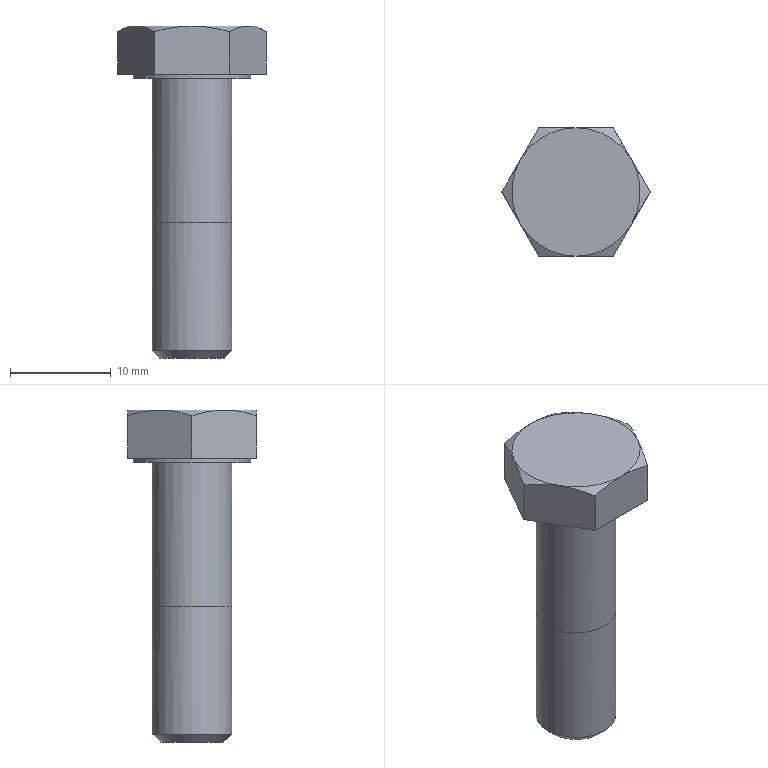Part | NX | features solid 2 | 1 solid | 20 faces | box 14.723 x 12.751 x 32.963 mm | volume 2081 mm3 | plane 10 | cone 7 | cylinder 3 | commonest cylinder face diameters 7.938 x2 11.684 x1
STEP:
#1=CARTESIAN_POINT('',(-3.969,0.,-5.182));
#2=VERTEX_POINT('',#1);
#3=CARTESIAN_POINT('',(0.,0.,-5.182));
#4=DIRECTION('',(0.,0.,-1.));
#5=DIRECTION('',(-1.,0.,0.));
#6=AXIS2_PLACEMENT_3D('',#3,#4,#5);
#7=CIRCLE('',#6,3.969);
#8=EDGE_CURVE('',#2,#2,#7,.T.);
#9=ORIENTED_EDGE('',*,*,#8,.T.);
#10=EDGE_LOOP('',(#9));
#11=FACE_BOUND('',#10,.T.);
#12=CARTESIAN_POINT('',(-3.969,0.,-19.469));
#13=VERTEX_POINT('',#12);
#14=CARTESIAN_POINT('',(-3.11,3.11,-19.469));
#15=CARTESIAN_POINT('',(-4.398,0.,-19.469));
#16=CARTESIAN_POINT('',(-3.11,-3.11,-19.469));
#17=CARTESIAN_POINT('',(0.,-4.398,-19.469));
#18=CARTESIAN_POINT('',(3.11,-3.11,-19.469));
#19=CARTESIAN_POINT('',(4.398,0.,-19.469));
#20=CARTESIAN_POINT('',(3.11,3.11,-19.469));
#21=CARTESIAN_POINT('',(0.,4.398,-19.469));
#22=CARTESIAN_POINT('',(-3.11,3.11,-19.469));
#23=CARTESIAN_POINT('',(-4.398,0.,-19.469));
#24=CARTESIAN_POINT('',(-3.11,-3.11,-19.469));
#25=B_SPLINE_CURVE_WITH_KNOTS('',3,(#14,#15,#16,#17,#18,#19,#20,#21,#22,#23,#24),.UNSPECIFIED.,.T.,.F.,(1,1,1,1,1,1,1,1,1,1,1,1,1,1,1),(-0.375,-0.25,-0.125,0.,0.125,0.25,0.375,0.5,0.625,0.75,0.875,1.,1.125,1.25,1.375),.UNSPECIFIED.);
#26=EDGE_CURVE('',#13,#13,#25,.T.);
#27=ORIENTED_EDGE('',*,*,#26,.T.);
#28=EDGE_LOOP('',(#27));
#29=FACE_BOUND('',#28,.T.);
#30=CARTESIAN_POINT('',(0.,0.,0.));
#31=DIRECTION('',(0.,0.,-1.));
#32=DIRECTION('',(-1.,0.,0.));
#33=AXIS2_PLACEMENT_3D('',#30,#31,#32);
#34=CYLINDRICAL_SURFACE('',#33,3.969);
#35=ADVANCED_FACE('',(#11,#29),#34,.T.);
#36=CARTESIAN_POINT('',(-7.362,0.,-4.775));
#37=VERTEX_POINT('',#36);
#38=CARTESIAN_POINT('',(-3.681,6.375,-4.775));
#39=VERTEX_POINT('',#38);
#40=CARTESIAN_POINT('',(-4.061,5.717,-4.775));
#41=DIRECTION('',(0.5,0.866,0.));
#42=VECTOR('',#41,1000.);
#43=LINE('',#40,#42);
#44=EDGE_CURVE('',#37,#39,#43,.T.);
#45=ORIENTED_EDGE('',*,*,#44,.T.);
#46=CARTESIAN_POINT('',(3.681,6.375,-4.775));
#47=VERTEX_POINT('',#46);
#48=CARTESIAN_POINT('',(5.842,6.375,-4.775));
#49=DIRECTION('',(1.,0.,0.));
#50=VECTOR('',#49,1000.);
#51=LINE('',#48,#50);
#52=EDGE_CURVE('',#39,#47,#51,.T.);
#53=ORIENTED_EDGE('',*,*,#52,.T.);
#54=CARTESIAN_POINT('',(7.362,0.,-4.775));
#55=VERTEX_POINT('',#54);
#56=CARTESIAN_POINT('',(6.982,0.658,-4.775));
#57=DIRECTION('',(0.5,-0.866,0.));
#58=VECTOR('',#57,1000.);
#59=LINE('',#56,#58);
#60=EDGE_CURVE('',#47,#55,#59,.T.);
#61=ORIENTED_EDGE('',*,*,#60,.T.);
#62=CARTESIAN_POINT('',(3.681,-6.375,-4.775));
#63=VERTEX_POINT('',#62);
#64=CARTESIAN_POINT('',(6.982,-0.658,-4.775));
#65=DIRECTION('',(-0.5,-0.866,0.));
#66=VECTOR('',#65,1000.);
#67=LINE('',#64,#66);
#68=EDGE_CURVE('',#55,#63,#67,.T.);
#69=ORIENTED_EDGE('',*,*,#68,.T.);
#70=CARTESIAN_POINT('',(-3.681,-6.375,-4.775));
#71=VERTEX_POINT('',#70);
#72=CARTESIAN_POINT('',(5.842,-6.375,-4.775));
#73=DIRECTION('',(-1.,0.,0.));
#74=VECTOR('',#73,1000.);
#75=LINE('',#72,#74);
#76=EDGE_CURVE('',#63,#71,#75,.T.);
#77=ORIENTED_EDGE('',*,*,#76,.T.);
#78=CARTESIAN_POINT('',(-4.061,-5.717,-4.775));
#79=DIRECTION('',(-0.5,0.866,0.));
#80=VECTOR('',#79,1000.);
#81=LINE('',#78,#80);
#82=EDGE_CURVE('',#71,#37,#81,.T.);
#83=ORIENTED_EDGE('',*,*,#82,.T.);
#84=EDGE_LOOP('',(#45,#53,#61,#69,#77,#83));
#85=FACE_BOUND('',#84,.T.);
#86=CARTESIAN_POINT('',(-5.842,0.,-4.775));
#87=VERTEX_POINT('',#86);
#88=CARTESIAN_POINT('',(0.,0.,-4.775));
#89=DIRECTION('',(0.,0.,-1.));
#90=DIRECTION('',(-1.,0.,0.));
#91=AXIS2_PLACEMENT_3D('',#88,#89,#90);
#92=CIRCLE('',#91,5.842);
#93=EDGE_CURVE('',#87,#87,#92,.T.);
#94=ORIENTED_EDGE('',*,*,#93,.F.);
#95=EDGE_LOOP('',(#94));
#96=FACE_BOUND('',#95,.T.);
#97=CARTESIAN_POINT('',(5.842,0.,-4.775));
#98=DIRECTION('',(0.,0.,-1.));
#99=DIRECTION('',(-1.,0.,0.));
#100=AXIS2_PLACEMENT_3D('',#97,#98,#99);
#101=PLANE('',#100);
#102=ADVANCED_FACE('',(#85,#96),#101,.T.);
#103=CARTESIAN_POINT('',(-3.181,0.,-32.963));
#104=VERTEX_POINT('',#103);
#105=CARTESIAN_POINT('',(0.,0.,-32.963));
#106=DIRECTION('',(0.,0.,-1.));
#107=DIRECTION('',(-1.,0.,0.));
#108=AXIS2_PLACEMENT_3D('',#105,#106,#107);
#109=CIRCLE('',#108,3.181);
#110=EDGE_CURVE('',#104,#104,#109,.T.);
#111=ORIENTED_EDGE('',*,*,#110,.T.);
#112=EDGE_LOOP('',(#111));
#113=FACE_BOUND('',#112,.T.);
#114=CARTESIAN_POINT('',(0.,0.,-32.963));
#115=DIRECTION('',(0.,0.,-1.));
#116=DIRECTION('',(-1.,0.,0.));
#117=AXIS2_PLACEMENT_3D('',#114,#115,#116);
#118=PLANE('',#117);
#119=ADVANCED_FACE('',(#113),#118,.T.);
#120=CARTESIAN_POINT('',(-3.969,0.,-32.175));
#121=VERTEX_POINT('',#120);
#122=CARTESIAN_POINT('',(0.,0.,-32.175));
#123=DIRECTION('',(0.,0.,-1.));
#124=DIRECTION('',(-1.,0.,0.));
#125=AXIS2_PLACEMENT_3D('',#122,#123,#124);
#126=CIRCLE('',#125,3.969);
#127=EDGE_CURVE('',#121,#121,#126,.T.);
#128=ORIENTED_EDGE('',*,*,#127,.T.);
#129=EDGE_LOOP('',(#128));
#130=FACE_BOUND('',#129,.T.);
#131=ORIENTED_EDGE('',*,*,#110,.F.);
#132=EDGE_LOOP('',(#131));
#133=FACE_BOUND('',#132,.T.);
#134=CARTESIAN_POINT('',(0.,0.,-32.963));
#135=DIRECTION('',(0.,0.,1.));
#136=DIRECTION('',(1.,0.,0.));
#137=AXIS2_PLACEMENT_3D('',#134,#135,#136);
#138=CONICAL_SURFACE('',#137,3.181,0.7854);
#139=ADVANCED_FACE('',(#130,#133),#138,.T.);
#140=ORIENTED_EDGE('',*,*,#26,.F.);
#141=EDGE_LOOP('',(#140));
#142=FACE_BOUND('',#141,.T.);
#143=ORIENTED_EDGE('',*,*,#127,.F.);
#144=EDGE_LOOP('',(#143));
#145=FACE_BOUND('',#144,.T.);
#146=CARTESIAN_POINT('',(0.,0.,0.));
#147=DIRECTION('',(0.,0.,-1.));
#148=DIRECTION('',(-1.,0.,0.));
#149=AXIS2_PLACEMENT_3D('',#146,#147,#148);
#150=CYLINDRICAL_SURFACE('',#149,3.969);
#151=ADVANCED_FACE('',(#142,#145),#150,.T.);
#152=CARTESIAN_POINT('',(-5.842,0.,-5.182));
#153=VERTEX_POINT('',#152);
#154=CARTESIAN_POINT('',(0.,0.,-5.182));
#155=DIRECTION('',(0.,0.,-1.));
#156=DIRECTION('',(-1.,0.,0.));
#157=AXIS2_PLACEMENT_3D('',#154,#155,#156);
#158=CIRCLE('',#157,5.842);
#159=EDGE_CURVE('',#153,#153,#158,.T.);
#160=ORIENTED_EDGE('',*,*,#159,.T.);
#161=EDGE_LOOP('',(#160));
#162=FACE_BOUND('',#161,.T.);
#163=ORIENTED_EDGE('',*,*,#8,.F.);
#164=EDGE_LOOP('',(#163));
#165=FACE_BOUND('',#164,.T.);
#166=CARTESIAN_POINT('',(3.969,0.,-5.182));
#167=DIRECTION('',(0.,0.,-1.));
#168=DIRECTION('',(-1.,0.,0.));
#169=AXIS2_PLACEMENT_3D('',#166,#167,#168);
#170=PLANE('',#169);
#171=ADVANCED_FACE('',(#162,#165),#170,.T.);
#172=ORIENTED_EDGE('',*,*,#93,.T.);
#173=EDGE_LOOP('',(#172));
#174=FACE_BOUND('',#173,.T.);
#175=ORIENTED_EDGE('',*,*,#159,.F.);
#176=EDGE_LOOP('',(#175));
#177=FACE_BOUND('',#176,.T.);
#178=CARTESIAN_POINT('',(0.,0.,0.));
#179=DIRECTION('',(0.,0.,-1.));
#180=DIRECTION('',(-1.,0.,0.));
#181=AXIS2_PLACEMENT_3D('',#178,#179,#180);
#182=CYLINDRICAL_SURFACE('',#181,5.842);
#183=ADVANCED_FACE('',(#174,#177),#182,.T.);
#184=ORIENTED_EDGE('',*,*,#52,.F.);
#185=CARTESIAN_POINT('',(-3.681,6.375,-0.5694));
#186=VERTEX_POINT('',#185);
#187=CARTESIAN_POINT('',(-3.681,6.375,-36.259));
#188=DIRECTION('',(0.,0.,1.));
#189=VECTOR('',#188,1000.);
#190=LINE('',#187,#189);
#191=EDGE_CURVE('',#39,#186,#190,.T.);
#192=ORIENTED_EDGE('',*,*,#191,.T.);
#193=CARTESIAN_POINT('',(0.,6.375,0.));
#194=VERTEX_POINT('',#193);
#195=CARTESIAN_POINT('',(-3.681,6.375,-0.5694));
#196=CARTESIAN_POINT('',(-2.484,6.375,-0.2238));
#197=CARTESIAN_POINT('',(-1.244,6.375,0.));
#198=CARTESIAN_POINT('',(0.,6.375,0.));
#199=B_SPLINE_CURVE_WITH_KNOTS('',3,(#195,#196,#197,#198),.UNSPECIFIED.,.F.,.F.,(4,4),(0.006567,0.01029),.UNSPECIFIED.);
#200=EDGE_CURVE('',#194,#186,#199,.F.);
#201=ORIENTED_EDGE('',*,*,#200,.F.);
#202=CARTESIAN_POINT('',(3.681,6.375,-0.5694));
#203=VERTEX_POINT('',#202);
#204=CARTESIAN_POINT('',(0.,6.375,0.));
#205=CARTESIAN_POINT('',(1.245,6.375,0.));
#206=CARTESIAN_POINT('',(2.49,6.375,-0.2258));
#207=CARTESIAN_POINT('',(3.681,6.375,-0.5694));
#208=B_SPLINE_CURVE_WITH_KNOTS('',3,(#204,#205,#206,#207),.UNSPECIFIED.,.F.,.F.,(4,4),(0.01029,0.01402),.UNSPECIFIED.);
#209=EDGE_CURVE('',#203,#194,#208,.F.);
#210=ORIENTED_EDGE('',*,*,#209,.F.);
#211=CARTESIAN_POINT('',(3.681,6.375,-36.259));
#212=DIRECTION('',(0.,0.,1.));
#213=VECTOR('',#212,1000.);
#214=LINE('',#211,#213);
#215=EDGE_CURVE('',#47,#203,#214,.T.);
#216=ORIENTED_EDGE('',*,*,#215,.F.);
#217=EDGE_LOOP('',(#184,#192,#201,#210,#216));
#218=FACE_BOUND('',#217,.T.);
#219=CARTESIAN_POINT('',(3.681,6.375,-36.259));
#220=DIRECTION('',(0.,1.,0.));
#221=DIRECTION('',(0.,0.,1.));
#222=AXIS2_PLACEMENT_3D('',#219,#220,#221);
#223=PLANE('',#222);
#224=ADVANCED_FACE('',(#218),#223,.T.);
#225=ORIENTED_EDGE('',*,*,#44,.F.);
#226=CARTESIAN_POINT('',(-7.362,0.,-0.5694));
#227=VERTEX_POINT('',#226);
#228=CARTESIAN_POINT('',(-7.362,0.,-36.259));
#229=DIRECTION('',(0.,0.,1.));
#230=VECTOR('',#229,1000.);
#231=LINE('',#228,#230);
#232=EDGE_CURVE('',#37,#227,#231,.T.);
#233=ORIENTED_EDGE('',*,*,#232,.T.);
#234=CARTESIAN_POINT('',(-5.521,3.188,0.));
#235=VERTEX_POINT('',#234);
#236=CARTESIAN_POINT('',(-5.521,3.188,0.));
#237=CARTESIAN_POINT('',(-6.146,2.106,0.));
#238=CARTESIAN_POINT('',(-6.761,1.04,-0.2227));
#239=CARTESIAN_POINT('',(-7.362,0.,-0.5694));
#240=B_SPLINE_CURVE_WITH_KNOTS('',3,(#236,#237,#238,#239),.UNSPECIFIED.,.F.,.F.,(4,4),(0.003725,0.007435),.UNSPECIFIED.);
#241=EDGE_CURVE('',#235,#227,#240,.T.);
#242=ORIENTED_EDGE('',*,*,#241,.F.);
#243=CARTESIAN_POINT('',(-3.681,6.375,-0.5694));
#244=CARTESIAN_POINT('',(-4.283,5.332,-0.2218));
#245=CARTESIAN_POINT('',(-4.894,4.274,0.));
#246=CARTESIAN_POINT('',(-5.521,3.188,0.));
#247=B_SPLINE_CURVE_WITH_KNOTS('',3,(#243,#244,#245,#246),.UNSPECIFIED.,.F.,.F.,(4,4),(0.000000238,0.003725),.UNSPECIFIED.);
#248=EDGE_CURVE('',#186,#235,#247,.T.);
#249=ORIENTED_EDGE('',*,*,#248,.F.);
#250=ORIENTED_EDGE('',*,*,#191,.F.);
#251=EDGE_LOOP('',(#225,#233,#242,#249,#250));
#252=FACE_BOUND('',#251,.T.);
#253=CARTESIAN_POINT('',(-3.681,6.375,-36.259));
#254=DIRECTION('',(-0.866,0.5,0.));
#255=DIRECTION('',(-0.5,-0.866,0.));
#256=AXIS2_PLACEMENT_3D('',#253,#254,#255);
#257=PLANE('',#256);
#258=ADVANCED_FACE('',(#252),#257,.T.);
#259=ORIENTED_EDGE('',*,*,#82,.F.);
#260=CARTESIAN_POINT('',(-3.681,-6.375,-0.5694));
#261=VERTEX_POINT('',#260);
#262=CARTESIAN_POINT('',(-3.681,-6.375,-36.259));
#263=DIRECTION('',(0.,0.,1.));
#264=VECTOR('',#263,1000.);
#265=LINE('',#262,#264);
#266=EDGE_CURVE('',#71,#261,#265,.T.);
#267=ORIENTED_EDGE('',*,*,#266,.T.);
#268=CARTESIAN_POINT('',(-5.521,-3.188,0.));
#269=VERTEX_POINT('',#268);
#270=CARTESIAN_POINT('',(-5.521,-3.188,0.));
#271=CARTESIAN_POINT('',(-4.896,-4.27,0.));
#272=CARTESIAN_POINT('',(-4.281,-5.335,-0.2227));
#273=CARTESIAN_POINT('',(-3.681,-6.375,-0.5694));
#274=B_SPLINE_CURVE_WITH_KNOTS('',3,(#270,#271,#272,#273),.UNSPECIFIED.,.F.,.F.,(4,4),(0.003725,0.007435),.UNSPECIFIED.);
#275=EDGE_CURVE('',#269,#261,#274,.T.);
#276=ORIENTED_EDGE('',*,*,#275,.F.);
#277=CARTESIAN_POINT('',(-7.362,0.,-0.5694));
#278=CARTESIAN_POINT('',(-6.76,-1.043,-0.2218));
#279=CARTESIAN_POINT('',(-6.148,-2.102,0.));
#280=CARTESIAN_POINT('',(-5.521,-3.188,0.));
#281=B_SPLINE_CURVE_WITH_KNOTS('',3,(#277,#278,#279,#280),.UNSPECIFIED.,.F.,.F.,(4,4),(0.000000238,0.003725),.UNSPECIFIED.);
#282=EDGE_CURVE('',#227,#269,#281,.T.);
#283=ORIENTED_EDGE('',*,*,#282,.F.);
#284=ORIENTED_EDGE('',*,*,#232,.F.);
#285=EDGE_LOOP('',(#259,#267,#276,#283,#284));
#286=FACE_BOUND('',#285,.T.);
#287=CARTESIAN_POINT('',(-7.362,0.,-36.259));
#288=DIRECTION('',(-0.866,-0.5,0.));
#289=DIRECTION('',(0.5,-0.866,0.));
#290=AXIS2_PLACEMENT_3D('',#287,#288,#289);
#291=PLANE('',#290);
#292=ADVANCED_FACE('',(#286),#291,.T.);
#293=ORIENTED_EDGE('',*,*,#76,.F.);
#294=CARTESIAN_POINT('',(3.681,-6.375,-0.5694));
#295=VERTEX_POINT('',#294);
#296=CARTESIAN_POINT('',(3.681,-6.375,-36.259));
#297=DIRECTION('',(0.,0.,1.));
#298=VECTOR('',#297,1000.);
#299=LINE('',#296,#298);
#300=EDGE_CURVE('',#63,#295,#299,.T.);
#301=ORIENTED_EDGE('',*,*,#300,.T.);
#302=CARTESIAN_POINT('',(0.,-6.375,0.));
#303=VERTEX_POINT('',#302);
#304=CARTESIAN_POINT('',(0.,-6.375,0.));
#305=CARTESIAN_POINT('',(1.245,-6.375,0.));
#306=CARTESIAN_POINT('',(2.49,-6.375,-0.2258));
#307=CARTESIAN_POINT('',(3.681,-6.375,-0.5694));
#308=B_SPLINE_CURVE_WITH_KNOTS('',3,(#304,#305,#306,#307),.UNSPECIFIED.,.F.,.F.,(4,4),(0.01029,0.01402),.UNSPECIFIED.);
#309=EDGE_CURVE('',#303,#295,#308,.T.);
#310=ORIENTED_EDGE('',*,*,#309,.F.);
#311=CARTESIAN_POINT('',(-3.681,-6.375,-0.5694));
#312=CARTESIAN_POINT('',(-2.484,-6.375,-0.2238));
#313=CARTESIAN_POINT('',(-1.244,-6.375,0.));
#314=CARTESIAN_POINT('',(0.,-6.375,0.));
#315=B_SPLINE_CURVE_WITH_KNOTS('',3,(#311,#312,#313,#314),.UNSPECIFIED.,.F.,.F.,(4,4),(0.006567,0.01029),.UNSPECIFIED.);
#316=EDGE_CURVE('',#261,#303,#315,.T.);
#317=ORIENTED_EDGE('',*,*,#316,.F.);
#318=ORIENTED_EDGE('',*,*,#266,.F.);
#319=EDGE_LOOP('',(#293,#301,#310,#317,#318));
#320=FACE_BOUND('',#319,.T.);
#321=CARTESIAN_POINT('',(-3.681,-6.375,-36.259));
#322=DIRECTION('',(0.,-1.,0.));
#323=DIRECTION('',(0.,0.,-1.));
#324=AXIS2_PLACEMENT_3D('',#321,#322,#323);
#325=PLANE('',#324);
#326=ADVANCED_FACE('',(#320),#325,.T.);
#327=ORIENTED_EDGE('',*,*,#68,.F.);
#328=CARTESIAN_POINT('',(7.362,0.,-0.5694));
#329=VERTEX_POINT('',#328);
#330=CARTESIAN_POINT('',(7.362,0.,-36.259));
#331=DIRECTION('',(0.,0.,1.));
#332=VECTOR('',#331,1000.);
#333=LINE('',#330,#332);
#334=EDGE_CURVE('',#55,#329,#333,.T.);
#335=ORIENTED_EDGE('',*,*,#334,.T.);
#336=CARTESIAN_POINT('',(5.521,-3.188,0.));
#337=VERTEX_POINT('',#336);
#338=CARTESIAN_POINT('',(5.521,-3.188,0.));
#339=CARTESIAN_POINT('',(6.146,-2.106,0.));
#340=CARTESIAN_POINT('',(6.761,-1.04,-0.2227));
#341=CARTESIAN_POINT('',(7.362,0.,-0.5694));
#342=B_SPLINE_CURVE_WITH_KNOTS('',3,(#338,#339,#340,#341),.UNSPECIFIED.,.F.,.F.,(4,4),(0.003725,0.007435),.UNSPECIFIED.);
#343=EDGE_CURVE('',#337,#329,#342,.T.);
#344=ORIENTED_EDGE('',*,*,#343,.F.);
#345=CARTESIAN_POINT('',(3.681,-6.375,-0.5694));
#346=CARTESIAN_POINT('',(4.283,-5.332,-0.2218));
#347=CARTESIAN_POINT('',(4.894,-4.274,0.));
#348=CARTESIAN_POINT('',(5.521,-3.188,0.));
#349=B_SPLINE_CURVE_WITH_KNOTS('',3,(#345,#346,#347,#348),.UNSPECIFIED.,.F.,.F.,(4,4),(0.000000238,0.003725),.UNSPECIFIED.);
#350=EDGE_CURVE('',#295,#337,#349,.T.);
#351=ORIENTED_EDGE('',*,*,#350,.F.);
#352=ORIENTED_EDGE('',*,*,#300,.F.);
#353=EDGE_LOOP('',(#327,#335,#344,#351,#352));
#354=FACE_BOUND('',#353,.T.);
#355=CARTESIAN_POINT('',(3.681,-6.375,-36.259));
#356=DIRECTION('',(0.866,-0.5,0.));
#357=DIRECTION('',(0.5,0.866,0.));
#358=AXIS2_PLACEMENT_3D('',#355,#356,#357);
#359=PLANE('',#358);
#360=ADVANCED_FACE('',(#354),#359,.T.);
#361=ORIENTED_EDGE('',*,*,#60,.F.);
#362=ORIENTED_EDGE('',*,*,#215,.T.);
#363=CARTESIAN_POINT('',(5.521,3.188,0.));
#364=VERTEX_POINT('',#363);
#365=CARTESIAN_POINT('',(5.521,3.188,0.));
#366=CARTESIAN_POINT('',(4.896,4.27,0.));
#367=CARTESIAN_POINT('',(4.281,5.335,-0.2227));
#368=CARTESIAN_POINT('',(3.681,6.375,-0.5694));
#369=B_SPLINE_CURVE_WITH_KNOTS('',3,(#365,#366,#367,#368),.UNSPECIFIED.,.F.,.F.,(4,4),(0.003725,0.007435),.UNSPECIFIED.);
#370=EDGE_CURVE('',#364,#203,#369,.T.);
#371=ORIENTED_EDGE('',*,*,#370,.F.);
#372=CARTESIAN_POINT('',(7.362,0.,-0.5694));
#373=CARTESIAN_POINT('',(6.76,1.043,-0.2218));
#374=CARTESIAN_POINT('',(6.148,2.102,0.));
#375=CARTESIAN_POINT('',(5.521,3.188,0.));
#376=B_SPLINE_CURVE_WITH_KNOTS('',3,(#372,#373,#374,#375),.UNSPECIFIED.,.F.,.F.,(4,4),(0.000000238,0.003725),.UNSPECIFIED.);
#377=EDGE_CURVE('',#329,#364,#376,.T.);
#378=ORIENTED_EDGE('',*,*,#377,.F.);
#379=ORIENTED_EDGE('',*,*,#334,.F.);
#380=EDGE_LOOP('',(#361,#362,#371,#378,#379));
#381=FACE_BOUND('',#380,.T.);
#382=CARTESIAN_POINT('',(7.362,0.,-36.259));
#383=DIRECTION('',(0.866,0.5,0.));
#384=DIRECTION('',(-0.5,0.866,0.));
#385=AXIS2_PLACEMENT_3D('',#382,#383,#384);
#386=PLANE('',#385);
#387=ADVANCED_FACE('',(#381),#386,.T.);
#388=CARTESIAN_POINT('',(0.,0.,0.));
#389=DIRECTION('',(0.,0.,-1.));
#390=DIRECTION('',(-1.,0.,0.));
#391=AXIS2_PLACEMENT_3D('',#388,#389,#390);
#392=CIRCLE('',#391,6.375);
#393=EDGE_CURVE('',#364,#337,#392,.T.);
#394=ORIENTED_EDGE('',*,*,#393,.T.);
#395=ORIENTED_EDGE('',*,*,#343,.T.);
#396=ORIENTED_EDGE('',*,*,#377,.T.);
#397=EDGE_LOOP('',(#394,#395,#396));
#398=FACE_BOUND('',#397,.T.);
#399=CARTESIAN_POINT('',(0.,0.,-0.5719));
#400=DIRECTION('',(0.,0.,-1.));
#401=DIRECTION('',(-1.,0.,0.));
#402=AXIS2_PLACEMENT_3D('',#399,#400,#401);
#403=CONICAL_SURFACE('',#402,7.366,1.047);
#404=ADVANCED_FACE('',(#398),#403,.T.);
#405=CARTESIAN_POINT('',(0.,0.,0.));
#406=DIRECTION('',(0.,0.,-1.));
#407=DIRECTION('',(-1.,0.,0.));
#408=AXIS2_PLACEMENT_3D('',#405,#406,#407);
#409=CIRCLE('',#408,6.375);
#410=EDGE_CURVE('',#337,#303,#409,.T.);
#411=ORIENTED_EDGE('',*,*,#410,.T.);
#412=ORIENTED_EDGE('',*,*,#309,.T.);
#413=ORIENTED_EDGE('',*,*,#350,.T.);
#414=EDGE_LOOP('',(#411,#412,#413));
#415=FACE_BOUND('',#414,.T.);
#416=CARTESIAN_POINT('',(0.,0.,-0.5719));
#417=DIRECTION('',(0.,0.,-1.));
#418=DIRECTION('',(-1.,0.,0.));
#419=AXIS2_PLACEMENT_3D('',#416,#417,#418);
#420=CONICAL_SURFACE('',#419,7.366,1.047);
#421=ADVANCED_FACE('',(#415),#420,.T.);
#422=CARTESIAN_POINT('',(0.,0.,0.));
#423=DIRECTION('',(0.,0.,-1.));
#424=DIRECTION('',(-1.,0.,0.));
#425=AXIS2_PLACEMENT_3D('',#422,#423,#424);
#426=CIRCLE('',#425,6.375);
#427=EDGE_CURVE('',#303,#269,#426,.T.);
#428=ORIENTED_EDGE('',*,*,#427,.T.);
#429=ORIENTED_EDGE('',*,*,#275,.T.);
#430=ORIENTED_EDGE('',*,*,#316,.T.);
#431=EDGE_LOOP('',(#428,#429,#430));
#432=FACE_BOUND('',#431,.T.);
#433=CARTESIAN_POINT('',(0.,0.,-0.5719));
#434=DIRECTION('',(0.,0.,-1.));
#435=DIRECTION('',(-1.,0.,0.));
#436=AXIS2_PLACEMENT_3D('',#433,#434,#435);
#437=CONICAL_SURFACE('',#436,7.366,1.047);
#438=ADVANCED_FACE('',(#432),#437,.T.);
#439=CARTESIAN_POINT('',(0.,0.,0.));
#440=DIRECTION('',(0.,0.,-1.));
#441=DIRECTION('',(-1.,0.,0.));
#442=AXIS2_PLACEMENT_3D('',#439,#440,#441);
#443=CIRCLE('',#442,6.375);
#444=EDGE_CURVE('',#269,#235,#443,.T.);
#445=ORIENTED_EDGE('',*,*,#444,.T.);
#446=ORIENTED_EDGE('',*,*,#241,.T.);
#447=ORIENTED_EDGE('',*,*,#282,.T.);
#448=EDGE_LOOP('',(#445,#446,#447));
#449=FACE_BOUND('',#448,.T.);
#450=CARTESIAN_POINT('',(0.,0.,-0.5719));
#451=DIRECTION('',(0.,0.,-1.));
#452=DIRECTION('',(-1.,0.,0.));
#453=AXIS2_PLACEMENT_3D('',#450,#451,#452);
#454=CONICAL_SURFACE('',#453,7.366,1.047);
#455=ADVANCED_FACE('',(#449),#454,.T.);
#456=CARTESIAN_POINT('',(0.,0.,0.));
#457=DIRECTION('',(0.,0.,-1.));
#458=DIRECTION('',(-1.,0.,0.));
#459=AXIS2_PLACEMENT_3D('',#456,#457,#458);
#460=CIRCLE('',#459,6.375);
#461=EDGE_CURVE('',#235,#194,#460,.T.);
#462=ORIENTED_EDGE('',*,*,#461,.T.);
#463=ORIENTED_EDGE('',*,*,#200,.T.);
#464=ORIENTED_EDGE('',*,*,#248,.T.);
#465=EDGE_LOOP('',(#462,#463,#464));
#466=FACE_BOUND('',#465,.T.);
#467=CARTESIAN_POINT('',(0.,0.,-0.5719));
#468=DIRECTION('',(0.,0.,-1.));
#469=DIRECTION('',(-1.,0.,0.));
#470=AXIS2_PLACEMENT_3D('',#467,#468,#469);
#471=CONICAL_SURFACE('',#470,7.366,1.047);
#472=ADVANCED_FACE('',(#466),#471,.T.);
#473=ORIENTED_EDGE('',*,*,#461,.F.);
#474=ORIENTED_EDGE('',*,*,#444,.F.);
#475=ORIENTED_EDGE('',*,*,#427,.F.);
#476=ORIENTED_EDGE('',*,*,#410,.F.);
#477=ORIENTED_EDGE('',*,*,#393,.F.);
#478=CARTESIAN_POINT('',(0.,0.,0.));
#479=DIRECTION('',(0.,0.,-1.));
#480=DIRECTION('',(-1.,0.,0.));
#481=AXIS2_PLACEMENT_3D('',#478,#479,#480);
#482=CIRCLE('',#481,6.375);
#483=EDGE_CURVE('',#194,#364,#482,.T.);
#484=ORIENTED_EDGE('',*,*,#483,.F.);
#485=EDGE_LOOP('',(#473,#474,#475,#476,#477,#484));
#486=FACE_BOUND('',#485,.T.);
#487=CARTESIAN_POINT('',(6.375,0.,0.));
#488=DIRECTION('',(0.,0.,1.));
#489=DIRECTION('',(1.,0.,0.));
#490=AXIS2_PLACEMENT_3D('',#487,#488,#489);
#491=PLANE('',#490);
#492=ADVANCED_FACE('',(#486),#491,.T.);
#493=ORIENTED_EDGE('',*,*,#370,.T.);
#494=ORIENTED_EDGE('',*,*,#209,.T.);
#495=ORIENTED_EDGE('',*,*,#483,.T.);
#496=EDGE_LOOP('',(#493,#494,#495));
#497=FACE_BOUND('',#496,.T.);
#498=CARTESIAN_POINT('',(0.,0.,-0.5719));
#499=DIRECTION('',(0.,0.,-1.));
#500=DIRECTION('',(-1.,0.,0.));
#501=AXIS2_PLACEMENT_3D('',#498,#499,#500);
#502=CONICAL_SURFACE('',#501,7.366,1.047);
#503=ADVANCED_FACE('',(#497),#502,.T.);
#504=CLOSED_SHELL('',(#35,#102,#119,#139,#151,#171,#183,#224,#258,#292,#326,#360,#387,#404,#421,#438,#455,#472,#492,#503));
#505=MANIFOLD_SOLID_BREP('',#504);
#506=(LENGTH_UNIT()NAMED_UNIT(*)SI_UNIT(.MILLI.,.METRE.));
#507=UNCERTAINTY_MEASURE_WITH_UNIT(LENGTH_MEASURE(0.0508),#506,'','');
#508=(NAMED_UNIT(*)PLANE_ANGLE_UNIT()SI_UNIT($,.RADIAN.));
#509=(NAMED_UNIT(*)SI_UNIT($,.STERADIAN.)SOLID_ANGLE_UNIT());
#510=(GEOMETRIC_REPRESENTATION_CONTEXT(3)GLOBAL_UNCERTAINTY_ASSIGNED_CONTEXT((#507))GLOBAL_UNIT_ASSIGNED_CONTEXT((#506,#508,#509))REPRESENTATION_CONTEXT('',''));
#511=ADVANCED_BREP_SHAPE_REPRESENTATION('',(#505),#510);